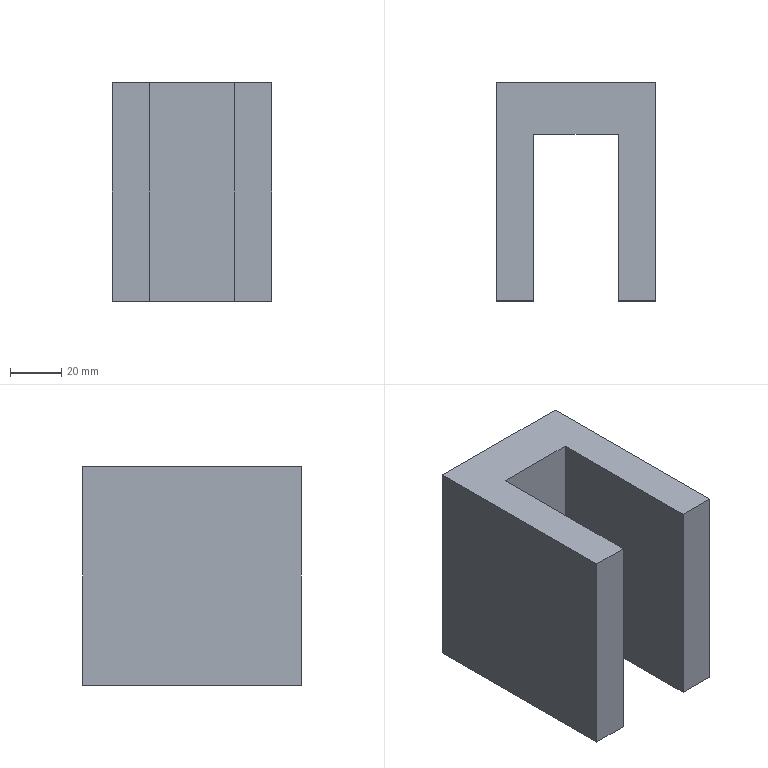Part | STEP file | BASE GUIA LINEAL_A | 1 solid | 10 faces | box 62 x 85 x 85 mm | volume 265625 mm3 | plane 10
STEP:
#1=CARTESIAN_POINT('',(16.5,0.,42.5));
#2=VERTEX_POINT('',#1);
#3=CARTESIAN_POINT('',(31.,0.,42.5));
#4=VERTEX_POINT('',#3);
#5=CARTESIAN_POINT('',(-31.,0.,42.5));
#6=DIRECTION('',(1.,0.,0.));
#7=VECTOR('',#6,1000.);
#8=LINE('',#5,#7);
#9=EDGE_CURVE('',#2,#4,#8,.T.);
#10=ORIENTED_EDGE('',*,*,#9,.F.);
#11=CARTESIAN_POINT('',(16.5,0.,-42.5));
#12=VERTEX_POINT('',#11);
#13=CARTESIAN_POINT('',(16.5,0.,42.5));
#14=DIRECTION('',(0.,0.,-1.));
#15=VECTOR('',#14,1000.);
#16=LINE('',#13,#15);
#17=EDGE_CURVE('',#2,#12,#16,.T.);
#18=ORIENTED_EDGE('',*,*,#17,.T.);
#19=CARTESIAN_POINT('',(31.,0.,-42.5));
#20=VERTEX_POINT('',#19);
#21=CARTESIAN_POINT('',(-31.,0.,-42.5));
#22=DIRECTION('',(1.,0.,0.));
#23=VECTOR('',#22,1000.);
#24=LINE('',#21,#23);
#25=EDGE_CURVE('',#12,#20,#24,.T.);
#26=ORIENTED_EDGE('',*,*,#25,.T.);
#27=CARTESIAN_POINT('',(31.,0.,42.5));
#28=DIRECTION('',(0.,0.,-1.));
#29=VECTOR('',#28,1000.);
#30=LINE('',#27,#29);
#31=EDGE_CURVE('',#4,#20,#30,.T.);
#32=ORIENTED_EDGE('',*,*,#31,.F.);
#33=EDGE_LOOP('',(#10,#18,#26,#32));
#34=FACE_OUTER_BOUND('',#33,.T.);
#35=CARTESIAN_POINT('',(-31.,0.,42.5));
#36=DIRECTION('',(0.,1.,0.));
#37=DIRECTION('',(-1.,0.,0.));
#38=AXIS2_PLACEMENT_3D('',#35,#36,#37);
#39=PLANE('',#38);
#40=ADVANCED_FACE('',(#34),#39,.F.);
#41=CARTESIAN_POINT('',(31.,85.,-42.5));
#42=VERTEX_POINT('',#41);
#43=CARTESIAN_POINT('',(31.,85.,-42.5));
#44=DIRECTION('',(0.,1.,0.));
#45=VECTOR('',#44,1000.);
#46=LINE('',#43,#45);
#47=EDGE_CURVE('',#20,#42,#46,.T.);
#48=ORIENTED_EDGE('',*,*,#47,.T.);
#49=CARTESIAN_POINT('',(31.,85.,42.5));
#50=VERTEX_POINT('',#49);
#51=CARTESIAN_POINT('',(31.,85.,42.5));
#52=DIRECTION('',(0.,0.,-1.));
#53=VECTOR('',#52,1000.);
#54=LINE('',#51,#53);
#55=EDGE_CURVE('',#50,#42,#54,.T.);
#56=ORIENTED_EDGE('',*,*,#55,.F.);
#57=CARTESIAN_POINT('',(31.,85.,42.5));
#58=DIRECTION('',(0.,1.,0.));
#59=VECTOR('',#58,1000.);
#60=LINE('',#57,#59);
#61=EDGE_CURVE('',#4,#50,#60,.T.);
#62=ORIENTED_EDGE('',*,*,#61,.F.);
#63=ORIENTED_EDGE('',*,*,#31,.T.);
#64=EDGE_LOOP('',(#48,#56,#62,#63));
#65=FACE_OUTER_BOUND('',#64,.T.);
#66=CARTESIAN_POINT('',(31.,85.,42.5));
#67=DIRECTION('',(-1.,0.,0.));
#68=DIRECTION('',(0.,0.,1.));
#69=AXIS2_PLACEMENT_3D('',#66,#67,#68);
#70=PLANE('',#69);
#71=ADVANCED_FACE('',(#65),#70,.F.);
#72=CARTESIAN_POINT('',(-31.,85.,-42.5));
#73=VERTEX_POINT('',#72);
#74=CARTESIAN_POINT('',(-31.,85.,-42.5));
#75=DIRECTION('',(-1.,0.,0.));
#76=VECTOR('',#75,1000.);
#77=LINE('',#74,#76);
#78=EDGE_CURVE('',#42,#73,#77,.T.);
#79=ORIENTED_EDGE('',*,*,#78,.T.);
#80=CARTESIAN_POINT('',(-31.,85.,42.5));
#81=VERTEX_POINT('',#80);
#82=CARTESIAN_POINT('',(-31.,85.,42.5));
#83=DIRECTION('',(0.,0.,-1.));
#84=VECTOR('',#83,1000.);
#85=LINE('',#82,#84);
#86=EDGE_CURVE('',#81,#73,#85,.T.);
#87=ORIENTED_EDGE('',*,*,#86,.F.);
#88=CARTESIAN_POINT('',(-31.,85.,42.5));
#89=DIRECTION('',(-1.,0.,0.));
#90=VECTOR('',#89,1000.);
#91=LINE('',#88,#90);
#92=EDGE_CURVE('',#50,#81,#91,.T.);
#93=ORIENTED_EDGE('',*,*,#92,.F.);
#94=ORIENTED_EDGE('',*,*,#55,.T.);
#95=EDGE_LOOP('',(#79,#87,#93,#94));
#96=FACE_OUTER_BOUND('',#95,.T.);
#97=CARTESIAN_POINT('',(-31.,85.,42.5));
#98=DIRECTION('',(0.,-1.,0.));
#99=DIRECTION('',(1.,0.,0.));
#100=AXIS2_PLACEMENT_3D('',#97,#98,#99);
#101=PLANE('',#100);
#102=ADVANCED_FACE('',(#96),#101,.F.);
#103=CARTESIAN_POINT('',(-31.,0.,-42.5));
#104=VERTEX_POINT('',#103);
#105=CARTESIAN_POINT('',(-31.,85.,-42.5));
#106=DIRECTION('',(0.,-1.,0.));
#107=VECTOR('',#106,1000.);
#108=LINE('',#105,#107);
#109=EDGE_CURVE('',#73,#104,#108,.T.);
#110=ORIENTED_EDGE('',*,*,#109,.T.);
#111=CARTESIAN_POINT('',(-31.,0.,42.5));
#112=VERTEX_POINT('',#111);
#113=CARTESIAN_POINT('',(-31.,0.,42.5));
#114=DIRECTION('',(0.,0.,-1.));
#115=VECTOR('',#114,1000.);
#116=LINE('',#113,#115);
#117=EDGE_CURVE('',#112,#104,#116,.T.);
#118=ORIENTED_EDGE('',*,*,#117,.F.);
#119=CARTESIAN_POINT('',(-31.,85.,42.5));
#120=DIRECTION('',(0.,-1.,0.));
#121=VECTOR('',#120,1000.);
#122=LINE('',#119,#121);
#123=EDGE_CURVE('',#81,#112,#122,.T.);
#124=ORIENTED_EDGE('',*,*,#123,.F.);
#125=ORIENTED_EDGE('',*,*,#86,.T.);
#126=EDGE_LOOP('',(#110,#118,#124,#125));
#127=FACE_OUTER_BOUND('',#126,.T.);
#128=CARTESIAN_POINT('',(-31.,85.,42.5));
#129=DIRECTION('',(1.,0.,0.));
#130=DIRECTION('',(0.,1.,0.));
#131=AXIS2_PLACEMENT_3D('',#128,#129,#130);
#132=PLANE('',#131);
#133=ADVANCED_FACE('',(#127),#132,.F.);
#134=CARTESIAN_POINT('',(-16.5,0.,-42.5));
#135=VERTEX_POINT('',#134);
#136=CARTESIAN_POINT('',(-31.,0.,-42.5));
#137=DIRECTION('',(1.,0.,0.));
#138=VECTOR('',#137,1000.);
#139=LINE('',#136,#138);
#140=EDGE_CURVE('',#104,#135,#139,.T.);
#141=ORIENTED_EDGE('',*,*,#140,.T.);
#142=CARTESIAN_POINT('',(-16.5,0.,42.5));
#143=VERTEX_POINT('',#142);
#144=CARTESIAN_POINT('',(-16.5,0.,42.5));
#145=DIRECTION('',(0.,0.,1.));
#146=VECTOR('',#145,1000.);
#147=LINE('',#144,#146);
#148=EDGE_CURVE('',#135,#143,#147,.T.);
#149=ORIENTED_EDGE('',*,*,#148,.T.);
#150=CARTESIAN_POINT('',(-31.,0.,42.5));
#151=DIRECTION('',(1.,0.,0.));
#152=VECTOR('',#151,1000.);
#153=LINE('',#150,#152);
#154=EDGE_CURVE('',#112,#143,#153,.T.);
#155=ORIENTED_EDGE('',*,*,#154,.F.);
#156=ORIENTED_EDGE('',*,*,#117,.T.);
#157=EDGE_LOOP('',(#141,#149,#155,#156));
#158=FACE_OUTER_BOUND('',#157,.T.);
#159=CARTESIAN_POINT('',(-31.,0.,42.5));
#160=DIRECTION('',(0.,1.,0.));
#161=DIRECTION('',(-1.,0.,0.));
#162=AXIS2_PLACEMENT_3D('',#159,#160,#161);
#163=PLANE('',#162);
#164=ADVANCED_FACE('',(#158),#163,.F.);
#165=CARTESIAN_POINT('',(16.5,65.,42.5));
#166=VERTEX_POINT('',#165);
#167=CARTESIAN_POINT('',(16.5,-65.,42.5));
#168=DIRECTION('',(0.,1.,0.));
#169=VECTOR('',#168,1000.);
#170=LINE('',#167,#169);
#171=EDGE_CURVE('',#2,#166,#170,.T.);
#172=ORIENTED_EDGE('',*,*,#171,.F.);
#173=ORIENTED_EDGE('',*,*,#9,.T.);
#174=ORIENTED_EDGE('',*,*,#61,.T.);
#175=ORIENTED_EDGE('',*,*,#92,.T.);
#176=ORIENTED_EDGE('',*,*,#123,.T.);
#177=ORIENTED_EDGE('',*,*,#154,.T.);
#178=CARTESIAN_POINT('',(-16.5,65.,42.5));
#179=VERTEX_POINT('',#178);
#180=CARTESIAN_POINT('',(-16.5,-65.,42.5));
#181=DIRECTION('',(0.,-1.,0.));
#182=VECTOR('',#181,1000.);
#183=LINE('',#180,#182);
#184=EDGE_CURVE('',#179,#143,#183,.T.);
#185=ORIENTED_EDGE('',*,*,#184,.F.);
#186=CARTESIAN_POINT('',(-16.5,65.,42.5));
#187=DIRECTION('',(-1.,0.,0.));
#188=VECTOR('',#187,1000.);
#189=LINE('',#186,#188);
#190=EDGE_CURVE('',#166,#179,#189,.T.);
#191=ORIENTED_EDGE('',*,*,#190,.F.);
#192=EDGE_LOOP('',(#172,#173,#174,#175,#176,#177,#185,#191));
#193=FACE_OUTER_BOUND('',#192,.T.);
#194=CARTESIAN_POINT('',(0.,0.,42.5));
#195=DIRECTION('',(0.,0.,1.));
#196=DIRECTION('',(1.,0.,0.));
#197=AXIS2_PLACEMENT_3D('',#194,#195,#196);
#198=PLANE('',#197);
#199=ADVANCED_FACE('',(#193),#198,.T.);
#200=ORIENTED_EDGE('',*,*,#25,.F.);
#201=CARTESIAN_POINT('',(16.5,65.,-42.5));
#202=VERTEX_POINT('',#201);
#203=CARTESIAN_POINT('',(16.5,0.,-42.5));
#204=DIRECTION('',(0.,1.,0.));
#205=VECTOR('',#204,1000.);
#206=LINE('',#203,#205);
#207=EDGE_CURVE('',#12,#202,#206,.T.);
#208=ORIENTED_EDGE('',*,*,#207,.T.);
#209=CARTESIAN_POINT('',(-16.5,65.,-42.5));
#210=VERTEX_POINT('',#209);
#211=CARTESIAN_POINT('',(-16.5,65.,-42.5));
#212=DIRECTION('',(-1.,0.,0.));
#213=VECTOR('',#212,1000.);
#214=LINE('',#211,#213);
#215=EDGE_CURVE('',#202,#210,#214,.T.);
#216=ORIENTED_EDGE('',*,*,#215,.T.);
#217=CARTESIAN_POINT('',(-16.5,-65.,-42.5));
#218=DIRECTION('',(0.,-1.,0.));
#219=VECTOR('',#218,1000.);
#220=LINE('',#217,#219);
#221=EDGE_CURVE('',#210,#135,#220,.T.);
#222=ORIENTED_EDGE('',*,*,#221,.T.);
#223=ORIENTED_EDGE('',*,*,#140,.F.);
#224=ORIENTED_EDGE('',*,*,#109,.F.);
#225=ORIENTED_EDGE('',*,*,#78,.F.);
#226=ORIENTED_EDGE('',*,*,#47,.F.);
#227=EDGE_LOOP('',(#200,#208,#216,#222,#223,#224,#225,#226));
#228=FACE_OUTER_BOUND('',#227,.T.);
#229=CARTESIAN_POINT('',(0.,0.,-42.5));
#230=DIRECTION('',(0.,0.,1.));
#231=DIRECTION('',(1.,0.,0.));
#232=AXIS2_PLACEMENT_3D('',#229,#230,#231);
#233=PLANE('',#232);
#234=ADVANCED_FACE('',(#228),#233,.F.);
#235=ORIENTED_EDGE('',*,*,#171,.T.);
#236=CARTESIAN_POINT('',(16.5,65.,-42.5));
#237=DIRECTION('',(0.,0.,1.));
#238=VECTOR('',#237,1000.);
#239=LINE('',#236,#238);
#240=EDGE_CURVE('',#202,#166,#239,.T.);
#241=ORIENTED_EDGE('',*,*,#240,.F.);
#242=ORIENTED_EDGE('',*,*,#207,.F.);
#243=ORIENTED_EDGE('',*,*,#17,.F.);
#244=EDGE_LOOP('',(#235,#241,#242,#243));
#245=FACE_OUTER_BOUND('',#244,.T.);
#246=CARTESIAN_POINT('',(16.5,-65.,-42.5));
#247=DIRECTION('',(1.,0.,0.));
#248=DIRECTION('',(0.,0.,-1.));
#249=AXIS2_PLACEMENT_3D('',#246,#247,#248);
#250=PLANE('',#249);
#251=ADVANCED_FACE('',(#245),#250,.F.);
#252=ORIENTED_EDGE('',*,*,#221,.F.);
#253=CARTESIAN_POINT('',(-16.5,65.,-42.5));
#254=DIRECTION('',(0.,0.,1.));
#255=VECTOR('',#254,1000.);
#256=LINE('',#253,#255);
#257=EDGE_CURVE('',#210,#179,#256,.T.);
#258=ORIENTED_EDGE('',*,*,#257,.T.);
#259=ORIENTED_EDGE('',*,*,#184,.T.);
#260=ORIENTED_EDGE('',*,*,#148,.F.);
#261=EDGE_LOOP('',(#252,#258,#259,#260));
#262=FACE_OUTER_BOUND('',#261,.T.);
#263=CARTESIAN_POINT('',(-16.5,-65.,-42.5));
#264=DIRECTION('',(-1.,0.,0.));
#265=DIRECTION('',(0.,0.,1.));
#266=AXIS2_PLACEMENT_3D('',#263,#264,#265);
#267=PLANE('',#266);
#268=ADVANCED_FACE('',(#262),#267,.F.);
#269=ORIENTED_EDGE('',*,*,#257,.F.);
#270=ORIENTED_EDGE('',*,*,#215,.F.);
#271=ORIENTED_EDGE('',*,*,#240,.T.);
#272=ORIENTED_EDGE('',*,*,#190,.T.);
#273=EDGE_LOOP('',(#269,#270,#271,#272));
#274=FACE_OUTER_BOUND('',#273,.T.);
#275=CARTESIAN_POINT('',(-16.5,65.,-42.5));
#276=DIRECTION('',(0.,1.,0.));
#277=DIRECTION('',(0.,0.,1.));
#278=AXIS2_PLACEMENT_3D('',#275,#276,#277);
#279=PLANE('',#278);
#280=ADVANCED_FACE('',(#274),#279,.F.);
#281=CLOSED_SHELL('',(#40,#71,#102,#133,#164,#199,#234,#251,#268,#280));
#282=MANIFOLD_SOLID_BREP('',#281);
#283=CARTESIAN_POINT('',(0.,0.,0.));
#284=DIRECTION('',(0.,0.,1.));
#285=DIRECTION('',(1.,0.,0.));
#286=AXIS2_PLACEMENT_3D('',#283,#284,#285);
#287=(LENGTH_UNIT()NAMED_UNIT(*)SI_UNIT(.MILLI.,.METRE.));
#288=UNCERTAINTY_MEASURE_WITH_UNIT(LENGTH_MEASURE(0.00001),#287,'','');
#289=(NAMED_UNIT(*)PLANE_ANGLE_UNIT()SI_UNIT($,.RADIAN.));
#290=(NAMED_UNIT(*)SI_UNIT($,.STERADIAN.)SOLID_ANGLE_UNIT());
#291=(GEOMETRIC_REPRESENTATION_CONTEXT(3)GLOBAL_UNCERTAINTY_ASSIGNED_CONTEXT((#288))GLOBAL_UNIT_ASSIGNED_CONTEXT((#287,#289,#290))REPRESENTATION_CONTEXT('',''));
#292=ADVANCED_BREP_SHAPE_REPRESENTATION('',(#282,#286),#291);